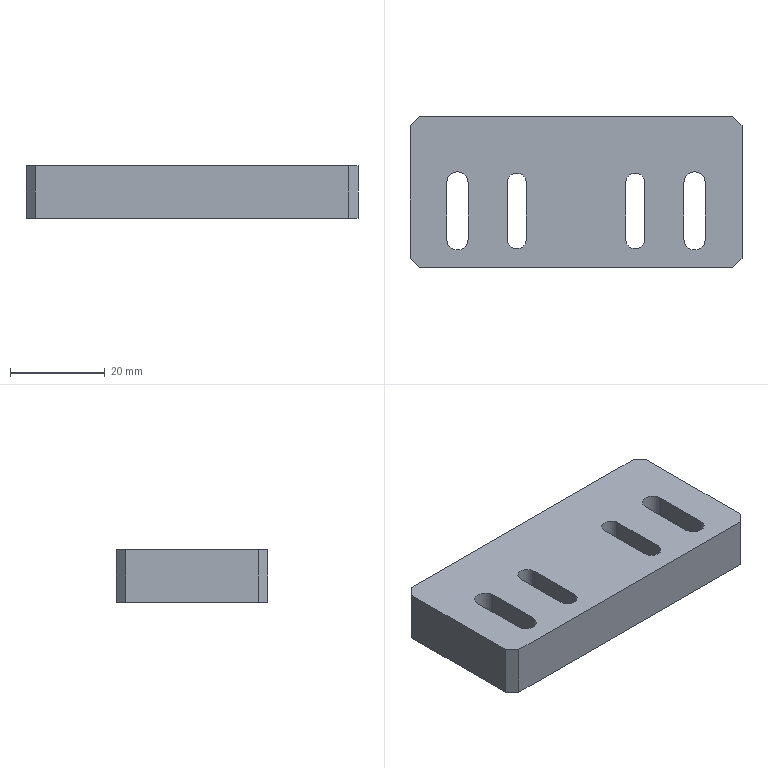Part | SolidWorks | features HoleWzd 4, Chamfer 1, Extrusion 1 | 1 solid | 46 faces | box 70 x 32 x 11 mm | volume 21010 mm3 | cylinder 18 | plane 18 | cone 10 | commonest cylinder face diameters 4 x8 4.2 x6 4.5 x4
STEP:
#1=CARTESIAN_POINT('',(-18.,10.,3.5));
#2=VERTEX_POINT('',#1);
#3=CARTESIAN_POINT('',(-18.,10.,7.5));
#4=VERTEX_POINT('',#3);
#5=CARTESIAN_POINT('',(-18.,10.,5.5));
#6=DIRECTION('',(0.,1.,0.));
#7=DIRECTION('',(0.,0.,1.));
#8=AXIS2_PLACEMENT_3D('',#5,#6,#7);
#9=CIRCLE('',#8,2.);
#10=EDGE_CURVE('',#2,#4,#9,.T.);
#11=ORIENTED_EDGE('',*,*,#10,.F.);
#12=CARTESIAN_POINT('',(-18.,16.,3.5));
#13=VERTEX_POINT('',#12);
#14=CARTESIAN_POINT('',(-18.,16.,3.5));
#15=DIRECTION('',(0.,1.,0.));
#16=VECTOR('',#15,1000.);
#17=LINE('',#14,#16);
#18=EDGE_CURVE('',#2,#13,#17,.T.);
#19=ORIENTED_EDGE('',*,*,#18,.T.);
#20=CARTESIAN_POINT('',(-18.,16.,7.5));
#21=VERTEX_POINT('',#20);
#22=CARTESIAN_POINT('',(-18.,16.,5.5));
#23=DIRECTION('',(0.,1.,0.));
#24=DIRECTION('',(0.,0.,1.));
#25=AXIS2_PLACEMENT_3D('',#22,#23,#24);
#26=CIRCLE('',#25,2.);
#27=EDGE_CURVE('',#13,#21,#26,.T.);
#28=ORIENTED_EDGE('',*,*,#27,.T.);
#29=CARTESIAN_POINT('',(-18.,16.,7.5));
#30=DIRECTION('',(0.,1.,0.));
#31=VECTOR('',#30,1000.);
#32=LINE('',#29,#31);
#33=EDGE_CURVE('',#4,#21,#32,.T.);
#34=ORIENTED_EDGE('',*,*,#33,.F.);
#35=EDGE_LOOP('',(#11,#19,#28,#34));
#36=FACE_OUTER_BOUND('',#35,.T.);
#37=CARTESIAN_POINT('',(-18.,16.,5.5));
#38=DIRECTION('',(0.,1.,0.));
#39=DIRECTION('',(0.,0.,1.));
#40=AXIS2_PLACEMENT_3D('',#37,#38,#39);
#41=CYLINDRICAL_SURFACE('',#40,2.);
#42=ADVANCED_FACE('',(#36),#41,.F.);
#43=CARTESIAN_POINT('',(-18.,8.798,5.5));
#44=VERTEX_POINT('',#43);
#45=CARTESIAN_POINT('',(-18.,10.,7.5));
#46=DIRECTION('',(0.,0.515,0.8572));
#47=VECTOR('',#46,1000.);
#48=LINE('',#45,#47);
#49=EDGE_CURVE('',#44,#4,#48,.T.);
#50=ORIENTED_EDGE('',*,*,#49,.F.);
#51=CARTESIAN_POINT('',(-18.,10.,3.5));
#52=DIRECTION('',(0.,0.515,-0.8572));
#53=VECTOR('',#52,1000.);
#54=LINE('',#51,#53);
#55=EDGE_CURVE('',#44,#2,#54,.T.);
#56=ORIENTED_EDGE('',*,*,#55,.T.);
#57=ORIENTED_EDGE('',*,*,#10,.T.);
#58=EDGE_LOOP('',(#50,#56,#57));
#59=FACE_OUTER_BOUND('',#58,.T.);
#60=CARTESIAN_POINT('',(-18.,10.,5.5));
#61=DIRECTION('',(0.,1.,0.));
#62=DIRECTION('',(0.,0.,1.));
#63=AXIS2_PLACEMENT_3D('',#60,#61,#62);
#64=CONICAL_SURFACE('',#63,2.,1.03);
#65=ADVANCED_FACE('',(#59),#64,.F.);
#66=CARTESIAN_POINT('',(18.,10.,3.5));
#67=VERTEX_POINT('',#66);
#68=CARTESIAN_POINT('',(18.,10.,7.5));
#69=VERTEX_POINT('',#68);
#70=CARTESIAN_POINT('',(18.,10.,5.5));
#71=DIRECTION('',(0.,1.,0.));
#72=DIRECTION('',(0.,0.,1.));
#73=AXIS2_PLACEMENT_3D('',#70,#71,#72);
#74=CIRCLE('',#73,2.);
#75=EDGE_CURVE('',#67,#69,#74,.T.);
#76=ORIENTED_EDGE('',*,*,#75,.F.);
#77=CARTESIAN_POINT('',(18.,16.,3.5));
#78=VERTEX_POINT('',#77);
#79=CARTESIAN_POINT('',(18.,16.,3.5));
#80=DIRECTION('',(0.,1.,0.));
#81=VECTOR('',#80,1000.);
#82=LINE('',#79,#81);
#83=EDGE_CURVE('',#67,#78,#82,.T.);
#84=ORIENTED_EDGE('',*,*,#83,.T.);
#85=CARTESIAN_POINT('',(18.,16.,7.5));
#86=VERTEX_POINT('',#85);
#87=CARTESIAN_POINT('',(18.,16.,5.5));
#88=DIRECTION('',(0.,1.,0.));
#89=DIRECTION('',(0.,0.,1.));
#90=AXIS2_PLACEMENT_3D('',#87,#88,#89);
#91=CIRCLE('',#90,2.);
#92=EDGE_CURVE('',#78,#86,#91,.T.);
#93=ORIENTED_EDGE('',*,*,#92,.T.);
#94=CARTESIAN_POINT('',(18.,16.,7.5));
#95=DIRECTION('',(0.,1.,0.));
#96=VECTOR('',#95,1000.);
#97=LINE('',#94,#96);
#98=EDGE_CURVE('',#69,#86,#97,.T.);
#99=ORIENTED_EDGE('',*,*,#98,.F.);
#100=EDGE_LOOP('',(#76,#84,#93,#99));
#101=FACE_OUTER_BOUND('',#100,.T.);
#102=CARTESIAN_POINT('',(18.,16.,5.5));
#103=DIRECTION('',(0.,1.,0.));
#104=DIRECTION('',(0.,0.,1.));
#105=AXIS2_PLACEMENT_3D('',#102,#103,#104);
#106=CYLINDRICAL_SURFACE('',#105,2.);
#107=ADVANCED_FACE('',(#101),#106,.F.);
#108=CARTESIAN_POINT('',(18.,8.798,5.5));
#109=VERTEX_POINT('',#108);
#110=CARTESIAN_POINT('',(18.,10.,7.5));
#111=DIRECTION('',(0.,0.515,0.8572));
#112=VECTOR('',#111,1000.);
#113=LINE('',#110,#112);
#114=EDGE_CURVE('',#109,#69,#113,.T.);
#115=ORIENTED_EDGE('',*,*,#114,.F.);
#116=CARTESIAN_POINT('',(18.,10.,3.5));
#117=DIRECTION('',(0.,0.515,-0.8572));
#118=VECTOR('',#117,1000.);
#119=LINE('',#116,#118);
#120=EDGE_CURVE('',#109,#67,#119,.T.);
#121=ORIENTED_EDGE('',*,*,#120,.T.);
#122=ORIENTED_EDGE('',*,*,#75,.T.);
#123=EDGE_LOOP('',(#115,#121,#122));
#124=FACE_OUTER_BOUND('',#123,.T.);
#125=CARTESIAN_POINT('',(18.,10.,5.5));
#126=DIRECTION('',(0.,1.,0.));
#127=DIRECTION('',(0.,0.,1.));
#128=AXIS2_PLACEMENT_3D('',#125,#126,#127);
#129=CONICAL_SURFACE('',#128,2.,1.03);
#130=ADVANCED_FACE('',(#124),#129,.F.);
#131=CARTESIAN_POINT('',(23.418,3.6,4.119));
#132=VERTEX_POINT('',#131);
#133=CARTESIAN_POINT('',(25.,4.25,3.4));
#134=VERTEX_POINT('',#133);
#135=CARTESIAN_POINT('',(23.418,3.6,4.119));
#136=CARTESIAN_POINT('',(23.508,3.688,4.016));
#137=CARTESIAN_POINT('',(23.607,3.772,3.922));
#138=CARTESIAN_POINT('',(23.83,3.927,3.75));
#139=CARTESIAN_POINT('',(23.955,3.998,3.672));
#140=CARTESIAN_POINT('',(24.225,4.117,3.542));
#141=CARTESIAN_POINT('',(24.371,4.166,3.49));
#142=CARTESIAN_POINT('',(24.68,4.233,3.418));
#143=CARTESIAN_POINT('',(24.838,4.25,3.4));
#144=CARTESIAN_POINT('',(25.,4.25,3.4));
#145=B_SPLINE_CURVE_WITH_KNOTS('',3,(#135,#136,#137,#138,#139,#140,#141,#142,#143,#144),.UNSPECIFIED.,.F.,.F.,(4,2,2,2,4),(0.,0.0004814,0.0009628,0.001444,0.001926),.UNSPECIFIED.);
#146=EDGE_CURVE('',#132,#134,#145,.T.);
#147=ORIENTED_EDGE('',*,*,#146,.T.);
#148=CARTESIAN_POINT('',(25.,16.,3.4));
#149=VERTEX_POINT('',#148);
#150=CARTESIAN_POINT('',(25.,16.,3.4));
#151=DIRECTION('',(0.,1.,0.));
#152=VECTOR('',#151,1000.);
#153=LINE('',#150,#152);
#154=EDGE_CURVE('',#134,#149,#153,.T.);
#155=ORIENTED_EDGE('',*,*,#154,.T.);
#156=CARTESIAN_POINT('',(25.,16.,7.6));
#157=VERTEX_POINT('',#156);
#158=CARTESIAN_POINT('',(25.,16.,5.5));
#159=DIRECTION('',(0.,1.,0.));
#160=DIRECTION('',(0.,0.,1.));
#161=AXIS2_PLACEMENT_3D('',#158,#159,#160);
#162=CIRCLE('',#161,2.1);
#163=EDGE_CURVE('',#149,#157,#162,.T.);
#164=ORIENTED_EDGE('',*,*,#163,.T.);
#165=CARTESIAN_POINT('',(25.,4.25,7.6));
#166=VERTEX_POINT('',#165);
#167=CARTESIAN_POINT('',(25.,16.,7.6));
#168=DIRECTION('',(0.,1.,0.));
#169=VECTOR('',#168,1000.);
#170=LINE('',#167,#169);
#171=EDGE_CURVE('',#166,#157,#170,.T.);
#172=ORIENTED_EDGE('',*,*,#171,.F.);
#173=CARTESIAN_POINT('',(23.418,3.6,6.881));
#174=VERTEX_POINT('',#173);
#175=CARTESIAN_POINT('',(25.,4.25,7.6));
#176=CARTESIAN_POINT('',(24.677,4.25,7.6));
#177=CARTESIAN_POINT('',(24.358,4.177,7.522));
#178=CARTESIAN_POINT('',(23.954,3.997,7.327));
#179=CARTESIAN_POINT('',(23.829,3.926,7.249));
#180=CARTESIAN_POINT('',(23.607,3.772,7.078));
#181=CARTESIAN_POINT('',(23.507,3.688,6.983));
#182=CARTESIAN_POINT('',(23.418,3.6,6.881));
#183=B_SPLINE_CURVE_WITH_KNOTS('',3,(#175,#176,#177,#178,#179,#180,#181,#182),.UNSPECIFIED.,.F.,.F.,(4,2,2,4),(0.001926,0.002886,0.003366,0.003846),.UNSPECIFIED.);
#184=EDGE_CURVE('',#166,#174,#183,.T.);
#185=ORIENTED_EDGE('',*,*,#184,.T.);
#186=CARTESIAN_POINT('',(25.,3.6,5.5));
#187=DIRECTION('',(0.,1.,0.));
#188=DIRECTION('',(0.,0.,1.));
#189=AXIS2_PLACEMENT_3D('',#186,#187,#188);
#190=CIRCLE('',#189,2.1);
#191=EDGE_CURVE('',#132,#174,#190,.T.);
#192=ORIENTED_EDGE('',*,*,#191,.F.);
#193=EDGE_LOOP('',(#147,#155,#164,#172,#185,#192));
#194=FACE_OUTER_BOUND('',#193,.T.);
#195=CARTESIAN_POINT('',(25.,16.,5.5));
#196=DIRECTION('',(0.,1.,0.));
#197=DIRECTION('',(0.,0.,1.));
#198=AXIS2_PLACEMENT_3D('',#195,#196,#197);
#199=CYLINDRICAL_SURFACE('',#198,2.1);
#200=ADVANCED_FACE('',(#194),#199,.F.);
#201=CARTESIAN_POINT('',(0.,3.6,3.4));
#202=VERTEX_POINT('',#201);
#203=CARTESIAN_POINT('',(0.,3.6,7.6));
#204=VERTEX_POINT('',#203);
#205=CARTESIAN_POINT('',(0.,3.6,5.5));
#206=DIRECTION('',(0.,1.,0.));
#207=DIRECTION('',(0.,0.,1.));
#208=AXIS2_PLACEMENT_3D('',#205,#206,#207);
#209=CIRCLE('',#208,2.1);
#210=EDGE_CURVE('',#202,#204,#209,.T.);
#211=ORIENTED_EDGE('',*,*,#210,.F.);
#212=CARTESIAN_POINT('',(0.,16.,3.4));
#213=VERTEX_POINT('',#212);
#214=CARTESIAN_POINT('',(0.,16.,3.4));
#215=DIRECTION('',(0.,1.,0.));
#216=VECTOR('',#215,1000.);
#217=LINE('',#214,#216);
#218=EDGE_CURVE('',#202,#213,#217,.T.);
#219=ORIENTED_EDGE('',*,*,#218,.T.);
#220=CARTESIAN_POINT('',(0.,16.,7.6));
#221=VERTEX_POINT('',#220);
#222=CARTESIAN_POINT('',(0.,16.,5.5));
#223=DIRECTION('',(0.,1.,0.));
#224=DIRECTION('',(0.,0.,1.));
#225=AXIS2_PLACEMENT_3D('',#222,#223,#224);
#226=CIRCLE('',#225,2.1);
#227=EDGE_CURVE('',#213,#221,#226,.T.);
#228=ORIENTED_EDGE('',*,*,#227,.T.);
#229=CARTESIAN_POINT('',(0.,16.,7.6));
#230=DIRECTION('',(0.,1.,0.));
#231=VECTOR('',#230,1000.);
#232=LINE('',#229,#231);
#233=EDGE_CURVE('',#204,#221,#232,.T.);
#234=ORIENTED_EDGE('',*,*,#233,.F.);
#235=EDGE_LOOP('',(#211,#219,#228,#234));
#236=FACE_OUTER_BOUND('',#235,.T.);
#237=CARTESIAN_POINT('',(0.,16.,5.5));
#238=DIRECTION('',(0.,1.,0.));
#239=DIRECTION('',(0.,0.,1.));
#240=AXIS2_PLACEMENT_3D('',#237,#238,#239);
#241=CYLINDRICAL_SURFACE('',#240,2.1);
#242=ADVANCED_FACE('',(#236),#241,.F.);
#243=CARTESIAN_POINT('',(0.,2.338,5.5));
#244=VERTEX_POINT('',#243);
#245=CARTESIAN_POINT('',(0.,3.6,7.6));
#246=DIRECTION('',(0.,0.515,0.8572));
#247=VECTOR('',#246,1000.);
#248=LINE('',#245,#247);
#249=EDGE_CURVE('',#244,#204,#248,.T.);
#250=ORIENTED_EDGE('',*,*,#249,.F.);
#251=CARTESIAN_POINT('',(0.,3.6,3.4));
#252=DIRECTION('',(0.,0.515,-0.8572));
#253=VECTOR('',#252,1000.);
#254=LINE('',#251,#253);
#255=EDGE_CURVE('',#244,#202,#254,.T.);
#256=ORIENTED_EDGE('',*,*,#255,.T.);
#257=ORIENTED_EDGE('',*,*,#210,.T.);
#258=EDGE_LOOP('',(#250,#256,#257));
#259=FACE_OUTER_BOUND('',#258,.T.);
#260=CARTESIAN_POINT('',(0.,3.6,5.5));
#261=DIRECTION('',(0.,1.,0.));
#262=DIRECTION('',(0.,0.,1.));
#263=AXIS2_PLACEMENT_3D('',#260,#261,#262);
#264=CONICAL_SURFACE('',#263,2.1,1.03);
#265=ADVANCED_FACE('',(#259),#264,.F.);
#266=CARTESIAN_POINT('',(-26.582,3.6,4.119));
#267=VERTEX_POINT('',#266);
#268=CARTESIAN_POINT('',(-25.,4.25,3.4));
#269=VERTEX_POINT('',#268);
#270=CARTESIAN_POINT('',(-26.582,3.6,4.119));
#271=CARTESIAN_POINT('',(-26.492,3.688,4.016));
#272=CARTESIAN_POINT('',(-26.393,3.772,3.922));
#273=CARTESIAN_POINT('',(-26.17,3.927,3.75));
#274=CARTESIAN_POINT('',(-26.045,3.998,3.672));
#275=CARTESIAN_POINT('',(-25.775,4.117,3.542));
#276=CARTESIAN_POINT('',(-25.629,4.166,3.49));
#277=CARTESIAN_POINT('',(-25.32,4.233,3.418));
#278=CARTESIAN_POINT('',(-25.162,4.25,3.4));
#279=CARTESIAN_POINT('',(-25.,4.25,3.4));
#280=B_SPLINE_CURVE_WITH_KNOTS('',3,(#270,#271,#272,#273,#274,#275,#276,#277,#278,#279),.UNSPECIFIED.,.F.,.F.,(4,2,2,2,4),(0.,0.0004814,0.0009628,0.001444,0.001926),.UNSPECIFIED.);
#281=EDGE_CURVE('',#267,#269,#280,.T.);
#282=ORIENTED_EDGE('',*,*,#281,.T.);
#283=CARTESIAN_POINT('',(-25.,16.,3.4));
#284=VERTEX_POINT('',#283);
#285=CARTESIAN_POINT('',(-25.,16.,3.4));
#286=DIRECTION('',(0.,1.,0.));
#287=VECTOR('',#286,1000.);
#288=LINE('',#285,#287);
#289=EDGE_CURVE('',#269,#284,#288,.T.);
#290=ORIENTED_EDGE('',*,*,#289,.T.);
#291=CARTESIAN_POINT('',(-25.,16.,7.6));
#292=VERTEX_POINT('',#291);
#293=CARTESIAN_POINT('',(-25.,16.,5.5));
#294=DIRECTION('',(0.,1.,0.));
#295=DIRECTION('',(0.,0.,1.));
#296=AXIS2_PLACEMENT_3D('',#293,#294,#295);
#297=CIRCLE('',#296,2.1);
#298=EDGE_CURVE('',#284,#292,#297,.T.);
#299=ORIENTED_EDGE('',*,*,#298,.T.);
#300=CARTESIAN_POINT('',(-25.,4.25,7.6));
#301=VERTEX_POINT('',#300);
#302=CARTESIAN_POINT('',(-25.,16.,7.6));
#303=DIRECTION('',(0.,1.,0.));
#304=VECTOR('',#303,1000.);
#305=LINE('',#302,#304);
#306=EDGE_CURVE('',#301,#292,#305,.T.);
#307=ORIENTED_EDGE('',*,*,#306,.F.);
#308=CARTESIAN_POINT('',(-26.582,3.6,6.881));
#309=VERTEX_POINT('',#308);
#310=CARTESIAN_POINT('',(-25.,4.25,7.6));
#311=CARTESIAN_POINT('',(-25.323,4.25,7.6));
#312=CARTESIAN_POINT('',(-25.642,4.177,7.522));
#313=CARTESIAN_POINT('',(-26.046,3.997,7.327));
#314=CARTESIAN_POINT('',(-26.171,3.926,7.249));
#315=CARTESIAN_POINT('',(-26.393,3.772,7.078));
#316=CARTESIAN_POINT('',(-26.493,3.688,6.983));
#317=CARTESIAN_POINT('',(-26.582,3.6,6.881));
#318=B_SPLINE_CURVE_WITH_KNOTS('',3,(#310,#311,#312,#313,#314,#315,#316,#317),.UNSPECIFIED.,.F.,.F.,(4,2,2,4),(0.001926,0.002886,0.003366,0.003846),.UNSPECIFIED.);
#319=EDGE_CURVE('',#301,#309,#318,.T.);
#320=ORIENTED_EDGE('',*,*,#319,.T.);
#321=CARTESIAN_POINT('',(-25.,3.6,5.5));
#322=DIRECTION('',(0.,1.,0.));
#323=DIRECTION('',(0.,0.,1.));
#324=AXIS2_PLACEMENT_3D('',#321,#322,#323);
#325=CIRCLE('',#324,2.1);
#326=EDGE_CURVE('',#267,#309,#325,.T.);
#327=ORIENTED_EDGE('',*,*,#326,.F.);
#328=EDGE_LOOP('',(#282,#290,#299,#307,#320,#327));
#329=FACE_OUTER_BOUND('',#328,.T.);
#330=CARTESIAN_POINT('',(-25.,16.,5.5));
#331=DIRECTION('',(0.,1.,0.));
#332=DIRECTION('',(0.,0.,1.));
#333=AXIS2_PLACEMENT_3D('',#330,#331,#332);
#334=CYLINDRICAL_SURFACE('',#333,2.1);
#335=ADVANCED_FACE('',(#329),#334,.F.);
#336=CARTESIAN_POINT('',(27.25,-10.,0.));
#337=VERTEX_POINT('',#336);
#338=CARTESIAN_POINT('',(27.25,2.,0.));
#339=VERTEX_POINT('',#338);
#340=CARTESIAN_POINT('',(27.25,-10.,0.));
#341=DIRECTION('',(0.,1.,0.));
#342=VECTOR('',#341,1000.);
#343=LINE('',#340,#342);
#344=EDGE_CURVE('',#337,#339,#343,.T.);
#345=ORIENTED_EDGE('',*,*,#344,.T.);
#346=CARTESIAN_POINT('',(22.75,2.,0.));
#347=VERTEX_POINT('',#346);
#348=CARTESIAN_POINT('',(25.,2.,0.));
#349=DIRECTION('',(0.,0.,-1.));
#350=DIRECTION('',(-1.,0.,0.));
#351=AXIS2_PLACEMENT_3D('',#348,#349,#350);
#352=CIRCLE('',#351,2.25);
#353=EDGE_CURVE('',#347,#339,#352,.T.);
#354=ORIENTED_EDGE('',*,*,#353,.F.);
#355=CARTESIAN_POINT('',(22.75,-10.,0.));
#356=VERTEX_POINT('',#355);
#357=CARTESIAN_POINT('',(22.75,-10.,0.));
#358=DIRECTION('',(0.,1.,0.));
#359=VECTOR('',#358,1000.);
#360=LINE('',#357,#359);
#361=EDGE_CURVE('',#356,#347,#360,.T.);
#362=ORIENTED_EDGE('',*,*,#361,.F.);
#363=CARTESIAN_POINT('',(25.,-10.,0.));
#364=DIRECTION('',(0.,0.,-1.));
#365=DIRECTION('',(-1.,0.,0.));
#366=AXIS2_PLACEMENT_3D('',#363,#364,#365);
#367=CIRCLE('',#366,2.25);
#368=EDGE_CURVE('',#337,#356,#367,.T.);
#369=ORIENTED_EDGE('',*,*,#368,.F.);
#370=EDGE_LOOP('',(#345,#354,#362,#369));
#371=FACE_BOUND('',#370,.T.);
#372=CARTESIAN_POINT('',(35.,-14.,0.));
#373=VERTEX_POINT('',#372);
#374=CARTESIAN_POINT('',(35.,14.,0.));
#375=VERTEX_POINT('',#374);
#376=CARTESIAN_POINT('',(35.,16.,0.));
#377=DIRECTION('',(0.,1.,0.));
#378=VECTOR('',#377,1000.);
#379=LINE('',#376,#378);
#380=EDGE_CURVE('',#373,#375,#379,.T.);
#381=ORIENTED_EDGE('',*,*,#380,.F.);
#382=CARTESIAN_POINT('',(33.,-16.,0.));
#383=VERTEX_POINT('',#382);
#384=CARTESIAN_POINT('',(35.,-14.,0.));
#385=DIRECTION('',(-0.7071,-0.7071,0.));
#386=VECTOR('',#385,1000.);
#387=LINE('',#384,#386);
#388=EDGE_CURVE('',#373,#383,#387,.T.);
#389=ORIENTED_EDGE('',*,*,#388,.T.);
#390=CARTESIAN_POINT('',(-33.,-16.,0.));
#391=VERTEX_POINT('',#390);
#392=CARTESIAN_POINT('',(-35.,-16.,0.));
#393=DIRECTION('',(1.,0.,0.));
#394=VECTOR('',#393,1000.);
#395=LINE('',#392,#394);
#396=EDGE_CURVE('',#391,#383,#395,.T.);
#397=ORIENTED_EDGE('',*,*,#396,.F.);
#398=CARTESIAN_POINT('',(-35.,-14.,0.));
#399=VERTEX_POINT('',#398);
#400=CARTESIAN_POINT('',(-33.,-16.,0.));
#401=DIRECTION('',(-0.7071,0.7071,0.));
#402=VECTOR('',#401,1000.);
#403=LINE('',#400,#402);
#404=EDGE_CURVE('',#391,#399,#403,.T.);
#405=ORIENTED_EDGE('',*,*,#404,.T.);
#406=CARTESIAN_POINT('',(-35.,14.,0.));
#407=VERTEX_POINT('',#406);
#408=CARTESIAN_POINT('',(-35.,16.,0.));
#409=DIRECTION('',(0.,-1.,0.));
#410=VECTOR('',#409,1000.);
#411=LINE('',#408,#410);
#412=EDGE_CURVE('',#407,#399,#411,.T.);
#413=ORIENTED_EDGE('',*,*,#412,.F.);
#414=CARTESIAN_POINT('',(-33.,16.,0.));
#415=VERTEX_POINT('',#414);
#416=CARTESIAN_POINT('',(-35.,14.,0.));
#417=DIRECTION('',(0.7071,0.7071,0.));
#418=VECTOR('',#417,1000.);
#419=LINE('',#416,#418);
#420=EDGE_CURVE('',#407,#415,#419,.T.);
#421=ORIENTED_EDGE('',*,*,#420,.T.);
#422=CARTESIAN_POINT('',(33.,16.,0.));
#423=VERTEX_POINT('',#422);
#424=CARTESIAN_POINT('',(-35.,16.,0.));
#425=DIRECTION('',(-1.,0.,0.));
#426=VECTOR('',#425,1000.);
#427=LINE('',#424,#426);
#428=EDGE_CURVE('',#423,#415,#427,.T.);
#429=ORIENTED_EDGE('',*,*,#428,.F.);
#430=CARTESIAN_POINT('',(33.,16.,0.));
#431=DIRECTION('',(0.7071,-0.7071,0.));
#432=VECTOR('',#431,1000.);
#433=LINE('',#430,#432);
#434=EDGE_CURVE('',#423,#375,#433,.T.);
#435=ORIENTED_EDGE('',*,*,#434,.T.);
#436=EDGE_LOOP('',(#381,#389,#397,#405,#413,#421,#429,#435));
#437=FACE_OUTER_BOUND('',#436,.T.);
#438=CARTESIAN_POINT('',(-27.25,2.,0.));
#439=VERTEX_POINT('',#438);
#440=CARTESIAN_POINT('',(-22.75,2.,0.));
#441=VERTEX_POINT('',#440);
#442=CARTESIAN_POINT('',(-25.,2.,0.));
#443=DIRECTION('',(0.,0.,-1.));
#444=DIRECTION('',(-1.,0.,0.));
#445=AXIS2_PLACEMENT_3D('',#442,#443,#444);
#446=CIRCLE('',#445,2.25);
#447=EDGE_CURVE('',#439,#441,#446,.T.);
#448=ORIENTED_EDGE('',*,*,#447,.F.);
#449=CARTESIAN_POINT('',(-27.25,-10.,0.));
#450=VERTEX_POINT('',#449);
#451=CARTESIAN_POINT('',(-27.25,-10.,0.));
#452=DIRECTION('',(0.,1.,0.));
#453=VECTOR('',#452,1000.);
#454=LINE('',#451,#453);
#455=EDGE_CURVE('',#450,#439,#454,.T.);
#456=ORIENTED_EDGE('',*,*,#455,.F.);
#457=CARTESIAN_POINT('',(-22.75,-10.,0.));
#458=VERTEX_POINT('',#457);
#459=CARTESIAN_POINT('',(-25.,-10.,0.));
#460=DIRECTION('',(0.,0.,-1.));
#461=DIRECTION('',(-1.,0.,0.));
#462=AXIS2_PLACEMENT_3D('',#459,#460,#461);
#463=CIRCLE('',#462,2.25);
#464=EDGE_CURVE('',#458,#450,#463,.T.);
#465=ORIENTED_EDGE('',*,*,#464,.F.);
#466=CARTESIAN_POINT('',(-22.75,-10.,0.));
#467=DIRECTION('',(0.,1.,0.));
#468=VECTOR('',#467,1000.);
#469=LINE('',#466,#468);
#470=EDGE_CURVE('',#458,#441,#469,.T.);
#471=ORIENTED_EDGE('',*,*,#470,.T.);
#472=EDGE_LOOP('',(#448,#456,#465,#471));
#473=FACE_BOUND('',#472,.T.);
#474=CARTESIAN_POINT('',(-14.5,2.,0.));
#475=VERTEX_POINT('',#474);
#476=CARTESIAN_POINT('',(-10.5,2.,0.));
#477=VERTEX_POINT('',#476);
#478=CARTESIAN_POINT('',(-12.5,2.,0.));
#479=DIRECTION('',(0.,0.,-1.));
#480=DIRECTION('',(-1.,0.,0.));
#481=AXIS2_PLACEMENT_3D('',#478,#479,#480);
#482=CIRCLE('',#481,2.);
#483=EDGE_CURVE('',#475,#477,#482,.T.);
#484=ORIENTED_EDGE('',*,*,#483,.F.);
#485=CARTESIAN_POINT('',(-14.5,-10.,0.));
#486=VERTEX_POINT('',#485);
#487=CARTESIAN_POINT('',(-14.5,-10.,0.));
#488=DIRECTION('',(0.,1.,0.));
#489=VECTOR('',#488,1000.);
#490=LINE('',#487,#489);
#491=EDGE_CURVE('',#486,#475,#490,.T.);
#492=ORIENTED_EDGE('',*,*,#491,.F.);
#493=CARTESIAN_POINT('',(-10.5,-10.,0.));
#494=VERTEX_POINT('',#493);
#495=CARTESIAN_POINT('',(-12.5,-10.,0.));
#496=DIRECTION('',(0.,0.,-1.));
#497=DIRECTION('',(-1.,0.,0.));
#498=AXIS2_PLACEMENT_3D('',#495,#496,#497);
#499=CIRCLE('',#498,2.);
#500=EDGE_CURVE('',#494,#486,#499,.T.);
#501=ORIENTED_EDGE('',*,*,#500,.F.);
#502=CARTESIAN_POINT('',(-10.5,-10.,0.));
#503=DIRECTION('',(0.,1.,0.));
#504=VECTOR('',#503,1000.);
#505=LINE('',#502,#504);
#506=EDGE_CURVE('',#494,#477,#505,.T.);
#507=ORIENTED_EDGE('',*,*,#506,.T.);
#508=EDGE_LOOP('',(#484,#492,#501,#507));
#509=FACE_BOUND('',#508,.T.);
#510=CARTESIAN_POINT('',(10.5,2.,0.));
#511=VERTEX_POINT('',#510);
#512=CARTESIAN_POINT('',(14.5,2.,0.));
#513=VERTEX_POINT('',#512);
#514=CARTESIAN_POINT('',(12.5,2.,0.));
#515=DIRECTION('',(0.,0.,-1.));
#516=DIRECTION('',(-1.,0.,0.));
#517=AXIS2_PLACEMENT_3D('',#514,#515,#516);
#518=CIRCLE('',#517,2.);
#519=EDGE_CURVE('',#511,#513,#518,.T.);
#520=ORIENTED_EDGE('',*,*,#519,.F.);
#521=CARTESIAN_POINT('',(10.5,-10.,0.));
#522=VERTEX_POINT('',#521);
#523=CARTESIAN_POINT('',(10.5,-10.,0.));
#524=DIRECTION('',(0.,1.,0.));
#525=VECTOR('',#524,1000.);
#526=LINE('',#523,#525);
#527=EDGE_CURVE('',#522,#511,#526,.T.);
#528=ORIENTED_EDGE('',*,*,#527,.F.);
#529=CARTESIAN_POINT('',(14.5,-10.,0.));
#530=VERTEX_POINT('',#529);
#531=CARTESIAN_POINT('',(12.5,-10.,0.));
#532=DIRECTION('',(0.,0.,-1.));
#533=DIRECTION('',(-1.,0.,0.));
#534=AXIS2_PLACEMENT_3D('',#531,#532,#533);
#535=CIRCLE('',#534,2.);
#536=EDGE_CURVE('',#530,#522,#535,.T.);
#537=ORIENTED_EDGE('',*,*,#536,.F.);
#538=CARTESIAN_POINT('',(14.5,-10.,0.));
#539=DIRECTION('',(0.,1.,0.));
#540=VECTOR('',#539,1000.);
#541=LINE('',#538,#540);
#542=EDGE_CURVE('',#530,#513,#541,.T.);
#543=ORIENTED_EDGE('',*,*,#542,.T.);
#544=EDGE_LOOP('',(#520,#528,#537,#543));
#545=FACE_BOUND('',#544,.T.);
#546=CARTESIAN_POINT('',(0.,0.,0.));
#547=DIRECTION('',(0.,0.,1.));
#548=DIRECTION('',(1.,0.,0.));
#549=AXIS2_PLACEMENT_3D('',#546,#547,#548);
#550=PLANE('',#549);
#551=ADVANCED_FACE('',(#371,#437,#473,#509,#545),#550,.F.);
#552=ORIENTED_EDGE('',*,*,#191,.T.);
#553=CARTESIAN_POINT('',(23.418,3.6,6.881));
#554=CARTESIAN_POINT('',(23.358,3.54,6.661));
#555=CARTESIAN_POINT('',(23.313,3.489,6.436));
#556=CARTESIAN_POINT('',(23.252,3.417,5.971));
#557=CARTESIAN_POINT('',(23.237,3.398,5.735));
#558=CARTESIAN_POINT('',(23.237,3.398,5.265));
#559=CARTESIAN_POINT('',(23.252,3.417,5.028));
#560=CARTESIAN_POINT('',(23.313,3.489,4.564));
#561=CARTESIAN_POINT('',(23.358,3.54,4.339));
#562=CARTESIAN_POINT('',(23.418,3.6,4.119));
#563=B_SPLINE_CURVE_WITH_KNOTS('',3,(#553,#554,#555,#556,#557,#558,#559,#560,#561,#562),.UNSPECIFIED.,.F.,.F.,(4,2,2,2,4),(0.000461,0.001167,0.001873,0.002579,0.003285),.UNSPECIFIED.);
#564=EDGE_CURVE('',#174,#132,#563,.T.);
#565=ORIENTED_EDGE('',*,*,#564,.T.);
#566=EDGE_LOOP('',(#552,#565));
#567=FACE_OUTER_BOUND('',#566,.T.);
#568=CARTESIAN_POINT('',(25.,3.6,5.5));
#569=DIRECTION('',(0.,1.,0.));
#570=DIRECTION('',(0.,0.,1.));
#571=AXIS2_PLACEMENT_3D('',#568,#569,#570);
#572=CONICAL_SURFACE('',#571,2.1,1.03);
#573=ADVANCED_FACE('',(#567),#572,.F.);
#574=ORIENTED_EDGE('',*,*,#326,.T.);
#575=CARTESIAN_POINT('',(-26.582,3.6,6.881));
#576=CARTESIAN_POINT('',(-26.642,3.54,6.661));
#577=CARTESIAN_POINT('',(-26.687,3.489,6.436));
#578=CARTESIAN_POINT('',(-26.748,3.417,5.971));
#579=CARTESIAN_POINT('',(-26.763,3.398,5.735));
#580=CARTESIAN_POINT('',(-26.763,3.398,5.265));
#581=CARTESIAN_POINT('',(-26.748,3.417,5.028));
#582=CARTESIAN_POINT('',(-26.687,3.489,4.564));
#583=CARTESIAN_POINT('',(-26.642,3.54,4.339));
#584=CARTESIAN_POINT('',(-26.582,3.6,4.119));
#585=B_SPLINE_CURVE_WITH_KNOTS('',3,(#575,#576,#577,#578,#579,#580,#581,#582,#583,#584),.UNSPECIFIED.,.F.,.F.,(4,2,2,2,4),(0.000461,0.001167,0.001873,0.002579,0.003285),.UNSPECIFIED.);
#586=EDGE_CURVE('',#309,#267,#585,.T.);
#587=ORIENTED_EDGE('',*,*,#586,.T.);
#588=EDGE_LOOP('',(#574,#587));
#589=FACE_OUTER_BOUND('',#588,.T.);
#590=CARTESIAN_POINT('',(-25.,3.6,5.5));
#591=DIRECTION('',(0.,1.,0.));
#592=DIRECTION('',(0.,0.,1.));
#593=AXIS2_PLACEMENT_3D('',#590,#591,#592);
#594=CONICAL_SURFACE('',#593,2.1,1.03);
#595=ADVANCED_FACE('',(#589),#594,.F.);
#596=CARTESIAN_POINT('',(35.,-14.,11.));
#597=VERTEX_POINT('',#596);
#598=CARTESIAN_POINT('',(35.,14.,11.));
#599=VERTEX_POINT('',#598);
#600=CARTESIAN_POINT('',(35.,16.,11.));
#601=DIRECTION('',(0.,1.,0.));
#602=VECTOR('',#601,1000.);
#603=LINE('',#600,#602);
#604=EDGE_CURVE('',#597,#599,#603,.T.);
#605=ORIENTED_EDGE('',*,*,#604,.F.);
#606=CARTESIAN_POINT('',(35.,-14.,11.));
#607=DIRECTION('',(0.,0.,-1.));
#608=VECTOR('',#607,1000.);
#609=LINE('',#606,#608);
#610=EDGE_CURVE('',#597,#373,#609,.T.);
#611=ORIENTED_EDGE('',*,*,#610,.T.);
#612=ORIENTED_EDGE('',*,*,#380,.T.);
#613=CARTESIAN_POINT('',(35.,14.,11.));
#614=DIRECTION('',(0.,0.,1.));
#615=VECTOR('',#614,1000.);
#616=LINE('',#613,#615);
#617=EDGE_CURVE('',#375,#599,#616,.T.);
#618=ORIENTED_EDGE('',*,*,#617,.T.);
#619=EDGE_LOOP('',(#605,#611,#612,#618));
#620=FACE_OUTER_BOUND('',#619,.T.);
#621=CARTESIAN_POINT('',(35.,16.,11.));
#622=DIRECTION('',(-1.,0.,0.));
#623=DIRECTION('',(0.,-1.,0.));
#624=AXIS2_PLACEMENT_3D('',#621,#622,#623);
#625=PLANE('',#624);
#626=ADVANCED_FACE('',(#620),#625,.F.);
#627=CARTESIAN_POINT('',(-18.,16.,5.5));
#628=DIRECTION('',(0.,1.,0.));
#629=DIRECTION('',(0.,0.,1.));
#630=AXIS2_PLACEMENT_3D('',#627,#628,#629);
#631=CIRCLE('',#630,2.);
#632=EDGE_CURVE('',#21,#13,#631,.T.);
#633=ORIENTED_EDGE('',*,*,#632,.F.);
#634=ORIENTED_EDGE('',*,*,#27,.F.);
#635=EDGE_LOOP('',(#633,#634));
#636=FACE_BOUND('',#635,.T.);
#637=CARTESIAN_POINT('',(18.,16.,5.5));
#638=DIRECTION('',(0.,1.,0.));
#639=DIRECTION('',(0.,0.,1.));
#640=AXIS2_PLACEMENT_3D('',#637,#638,#639);
#641=CIRCLE('',#640,2.);
#642=EDGE_CURVE('',#86,#78,#641,.T.);
#643=ORIENTED_EDGE('',*,*,#642,.F.);
#644=ORIENTED_EDGE('',*,*,#92,.F.);
#645=EDGE_LOOP('',(#643,#644));
#646=FACE_BOUND('',#645,.T.);
#647=CARTESIAN_POINT('',(25.,16.,5.5));
#648=DIRECTION('',(0.,1.,0.));
#649=DIRECTION('',(0.,0.,1.));
#650=AXIS2_PLACEMENT_3D('',#647,#648,#649);
#651=CIRCLE('',#650,2.1);
#652=EDGE_CURVE('',#157,#149,#651,.T.);
#653=ORIENTED_EDGE('',*,*,#652,.F.);
#654=ORIENTED_EDGE('',*,*,#163,.F.);
#655=EDGE_LOOP('',(#653,#654));
#656=FACE_BOUND('',#655,.T.);
#657=CARTESIAN_POINT('',(0.,16.,5.5));
#658=DIRECTION('',(0.,1.,0.));
#659=DIRECTION('',(0.,0.,1.));
#660=AXIS2_PLACEMENT_3D('',#657,#658,#659);
#661=CIRCLE('',#660,2.1);
#662=EDGE_CURVE('',#221,#213,#661,.T.);
#663=ORIENTED_EDGE('',*,*,#662,.F.);
#664=ORIENTED_EDGE('',*,*,#227,.F.);
#665=EDGE_LOOP('',(#663,#664));
#666=FACE_BOUND('',#665,.T.);
#667=CARTESIAN_POINT('',(-25.,16.,5.5));
#668=DIRECTION('',(0.,1.,0.));
#669=DIRECTION('',(0.,0.,1.));
#670=AXIS2_PLACEMENT_3D('',#667,#668,#669);
#671=CIRCLE('',#670,2.1);
#672=EDGE_CURVE('',#292,#284,#671,.T.);
#673=ORIENTED_EDGE('',*,*,#672,.F.);
#674=ORIENTED_EDGE('',*,*,#298,.F.);
#675=EDGE_LOOP('',(#673,#674));
#676=FACE_BOUND('',#675,.T.);
#677=CARTESIAN_POINT('',(33.,16.,11.));
#678=VERTEX_POINT('',#677);
#679=CARTESIAN_POINT('',(-33.,16.,11.));
#680=VERTEX_POINT('',#679);
#681=CARTESIAN_POINT('',(-35.,16.,11.));
#682=DIRECTION('',(-1.,0.,0.));
#683=VECTOR('',#682,1000.);
#684=LINE('',#681,#683);
#685=EDGE_CURVE('',#678,#680,#684,.T.);
#686=ORIENTED_EDGE('',*,*,#685,.F.);
#687=CARTESIAN_POINT('',(33.,16.,11.));
#688=DIRECTION('',(0.,0.,-1.));
#689=VECTOR('',#688,1000.);
#690=LINE('',#687,#689);
#691=EDGE_CURVE('',#678,#423,#690,.T.);
#692=ORIENTED_EDGE('',*,*,#691,.T.);
#693=ORIENTED_EDGE('',*,*,#428,.T.);
#694=CARTESIAN_POINT('',(-33.,16.,11.));
#695=DIRECTION('',(0.,0.,1.));
#696=VECTOR('',#695,1000.);
#697=LINE('',#694,#696);
#698=EDGE_CURVE('',#415,#680,#697,.T.);
#699=ORIENTED_EDGE('',*,*,#698,.T.);
#700=EDGE_LOOP('',(#686,#692,#693,#699));
#701=FACE_OUTER_BOUND('',#700,.T.);
#702=CARTESIAN_POINT('',(-35.,16.,11.));
#703=DIRECTION('',(0.,-1.,0.));
#704=DIRECTION('',(0.,0.,-1.));
#705=AXIS2_PLACEMENT_3D('',#702,#703,#704);
#706=PLANE('',#705);
#707=ADVANCED_FACE('',(#636,#646,#656,#666,#676,#701),#706,.F.);
#708=CARTESIAN_POINT('',(-35.,14.,11.));
#709=VERTEX_POINT('',#708);
#710=CARTESIAN_POINT('',(-35.,-14.,11.));
#711=VERTEX_POINT('',#710);
#712=CARTESIAN_POINT('',(-35.,16.,11.));
#713=DIRECTION('',(0.,-1.,0.));
#714=VECTOR('',#713,1000.);
#715=LINE('',#712,#714);
#716=EDGE_CURVE('',#709,#711,#715,.T.);
#717=ORIENTED_EDGE('',*,*,#716,.F.);
#718=CARTESIAN_POINT('',(-35.,14.,11.));
#719=DIRECTION('',(0.,0.,-1.));
#720=VECTOR('',#719,1000.);
#721=LINE('',#718,#720);
#722=EDGE_CURVE('',#709,#407,#721,.T.);
#723=ORIENTED_EDGE('',*,*,#722,.T.);
#724=ORIENTED_EDGE('',*,*,#412,.T.);
#725=CARTESIAN_POINT('',(-35.,-14.,11.));
#726=DIRECTION('',(0.,0.,1.));
#727=VECTOR('',#726,1000.);
#728=LINE('',#725,#727);
#729=EDGE_CURVE('',#399,#711,#728,.T.);
#730=ORIENTED_EDGE('',*,*,#729,.T.);
#731=EDGE_LOOP('',(#717,#723,#724,#730));
#732=FACE_OUTER_BOUND('',#731,.T.);
#733=CARTESIAN_POINT('',(-35.,16.,11.));
#734=DIRECTION('',(1.,0.,0.));
#735=DIRECTION('',(0.,1.,0.));
#736=AXIS2_PLACEMENT_3D('',#733,#734,#735);
#737=PLANE('',#736);
#738=ADVANCED_FACE('',(#732),#737,.F.);
#739=ORIENTED_EDGE('',*,*,#396,.T.);
#740=CARTESIAN_POINT('',(33.,-16.,11.));
#741=VERTEX_POINT('',#740);
#742=CARTESIAN_POINT('',(33.,-16.,11.));
#743=DIRECTION('',(0.,0.,1.));
#744=VECTOR('',#743,1000.);
#745=LINE('',#742,#744);
#746=EDGE_CURVE('',#383,#741,#745,.T.);
#747=ORIENTED_EDGE('',*,*,#746,.T.);
#748=CARTESIAN_POINT('',(-33.,-16.,11.));
#749=VERTEX_POINT('',#748);
#750=CARTESIAN_POINT('',(-35.,-16.,11.));
#751=DIRECTION('',(1.,0.,0.));
#752=VECTOR('',#751,1000.);
#753=LINE('',#750,#752);
#754=EDGE_CURVE('',#749,#741,#753,.T.);
#755=ORIENTED_EDGE('',*,*,#754,.F.);
#756=CARTESIAN_POINT('',(-33.,-16.,11.));
#757=DIRECTION('',(0.,0.,-1.));
#758=VECTOR('',#757,1000.);
#759=LINE('',#756,#758);
#760=EDGE_CURVE('',#749,#391,#759,.T.);
#761=ORIENTED_EDGE('',*,*,#760,.T.);
#762=EDGE_LOOP('',(#739,#747,#755,#761));
#763=FACE_OUTER_BOUND('',#762,.T.);
#764=CARTESIAN_POINT('',(-35.,-16.,11.));
#765=DIRECTION('',(0.,1.,0.));
#766=DIRECTION('',(0.,0.,1.));
#767=AXIS2_PLACEMENT_3D('',#764,#765,#766);
#768=PLANE('',#767);
#769=ADVANCED_FACE('',(#763),#768,.F.);
#770=CARTESIAN_POINT('',(14.5,2.,11.));
#771=VERTEX_POINT('',#770);
#772=CARTESIAN_POINT('',(10.5,2.,11.));
#773=VERTEX_POINT('',#772);
#774=CARTESIAN_POINT('',(12.5,2.,11.));
#775=DIRECTION('',(0.,0.,1.));
#776=DIRECTION('',(1.,0.,0.));
#777=AXIS2_PLACEMENT_3D('',#774,#775,#776);
#778=CIRCLE('',#777,2.);
#779=EDGE_CURVE('',#771,#773,#778,.T.);
#780=ORIENTED_EDGE('',*,*,#779,.F.);
#781=CARTESIAN_POINT('',(14.5,-10.,11.));
#782=VERTEX_POINT('',#781);
#783=CARTESIAN_POINT('',(14.5,0.,11.));
#784=DIRECTION('',(0.,-1.,0.));
#785=VECTOR('',#784,1000.);
#786=LINE('',#783,#785);
#787=EDGE_CURVE('',#771,#782,#786,.T.);
#788=ORIENTED_EDGE('',*,*,#787,.T.);
#789=CARTESIAN_POINT('',(10.5,-10.,11.));
#790=VERTEX_POINT('',#789);
#791=CARTESIAN_POINT('',(12.5,-10.,11.));
#792=DIRECTION('',(0.,0.,1.));
#793=DIRECTION('',(1.,0.,0.));
#794=AXIS2_PLACEMENT_3D('',#791,#792,#793);
#795=CIRCLE('',#794,2.);
#796=EDGE_CURVE('',#790,#782,#795,.T.);
#797=ORIENTED_EDGE('',*,*,#796,.F.);
#798=CARTESIAN_POINT('',(10.5,0.,11.));
#799=DIRECTION('',(0.,-1.,0.));
#800=VECTOR('',#799,1000.);
#801=LINE('',#798,#800);
#802=EDGE_CURVE('',#773,#790,#801,.T.);
#803=ORIENTED_EDGE('',*,*,#802,.F.);
#804=EDGE_LOOP('',(#780,#788,#797,#803));
#805=FACE_BOUND('',#804,.T.);
#806=CARTESIAN_POINT('',(-14.5,-10.,11.));
#807=VERTEX_POINT('',#806);
#808=CARTESIAN_POINT('',(-10.5,-10.,11.));
#809=VERTEX_POINT('',#808);
#810=CARTESIAN_POINT('',(-12.5,-10.,11.));
#811=DIRECTION('',(0.,0.,1.));
#812=DIRECTION('',(1.,0.,0.));
#813=AXIS2_PLACEMENT_3D('',#810,#811,#812);
#814=CIRCLE('',#813,2.);
#815=EDGE_CURVE('',#807,#809,#814,.T.);
#816=ORIENTED_EDGE('',*,*,#815,.F.);
#817=CARTESIAN_POINT('',(-14.5,2.,11.));
#818=VERTEX_POINT('',#817);
#819=CARTESIAN_POINT('',(-14.5,0.,11.));
#820=DIRECTION('',(0.,-1.,0.));
#821=VECTOR('',#820,1000.);
#822=LINE('',#819,#821);
#823=EDGE_CURVE('',#818,#807,#822,.T.);
#824=ORIENTED_EDGE('',*,*,#823,.F.);
#825=CARTESIAN_POINT('',(-10.5,2.,11.));
#826=VERTEX_POINT('',#825);
#827=CARTESIAN_POINT('',(-12.5,2.,11.));
#828=DIRECTION('',(0.,0.,1.));
#829=DIRECTION('',(1.,0.,0.));
#830=AXIS2_PLACEMENT_3D('',#827,#828,#829);
#831=CIRCLE('',#830,2.);
#832=EDGE_CURVE('',#826,#818,#831,.T.);
#833=ORIENTED_EDGE('',*,*,#832,.F.);
#834=CARTESIAN_POINT('',(-10.5,0.,11.));
#835=DIRECTION('',(0.,-1.,0.));
#836=VECTOR('',#835,1000.);
#837=LINE('',#834,#836);
#838=EDGE_CURVE('',#826,#809,#837,.T.);
#839=ORIENTED_EDGE('',*,*,#838,.T.);
#840=EDGE_LOOP('',(#816,#824,#833,#839));
#841=FACE_BOUND('',#840,.T.);
#842=CARTESIAN_POINT('',(22.75,-10.,11.));
#843=VERTEX_POINT('',#842);
#844=CARTESIAN_POINT('',(27.25,-10.,11.));
#845=VERTEX_POINT('',#844);
#846=CARTESIAN_POINT('',(25.,-10.,11.));
#847=DIRECTION('',(0.,0.,1.));
#848=DIRECTION('',(1.,0.,0.));
#849=AXIS2_PLACEMENT_3D('',#846,#847,#848);
#850=CIRCLE('',#849,2.25);
#851=EDGE_CURVE('',#843,#845,#850,.T.);
#852=ORIENTED_EDGE('',*,*,#851,.F.);
#853=CARTESIAN_POINT('',(22.75,2.,11.));
#854=VERTEX_POINT('',#853);
#855=CARTESIAN_POINT('',(22.75,0.,11.));
#856=DIRECTION('',(0.,-1.,0.));
#857=VECTOR('',#856,1000.);
#858=LINE('',#855,#857);
#859=EDGE_CURVE('',#854,#843,#858,.T.);
#860=ORIENTED_EDGE('',*,*,#859,.F.);
#861=CARTESIAN_POINT('',(27.25,2.,11.));
#862=VERTEX_POINT('',#861);
#863=CARTESIAN_POINT('',(25.,2.,11.));
#864=DIRECTION('',(0.,0.,1.));
#865=DIRECTION('',(1.,0.,0.));
#866=AXIS2_PLACEMENT_3D('',#863,#864,#865);
#867=CIRCLE('',#866,2.25);
#868=EDGE_CURVE('',#862,#854,#867,.T.);
#869=ORIENTED_EDGE('',*,*,#868,.F.);
#870=CARTESIAN_POINT('',(27.25,0.,11.));
#871=DIRECTION('',(0.,-1.,0.));
#872=VECTOR('',#871,1000.);
#873=LINE('',#870,#872);
#874=EDGE_CURVE('',#862,#845,#873,.T.);
#875=ORIENTED_EDGE('',*,*,#874,.T.);
#876=EDGE_LOOP('',(#852,#860,#869,#875));
#877=FACE_BOUND('',#876,.T.);
#878=CARTESIAN_POINT('',(-27.25,2.,11.));
#879=VERTEX_POINT('',#878);
#880=CARTESIAN_POINT('',(-27.25,-10.,11.));
#881=VERTEX_POINT('',#880);
#882=CARTESIAN_POINT('',(-27.25,0.,11.));
#883=DIRECTION('',(0.,-1.,0.));
#884=VECTOR('',#883,1000.);
#885=LINE('',#882,#884);
#886=EDGE_CURVE('',#879,#881,#885,.T.);
#887=ORIENTED_EDGE('',*,*,#886,.F.);
#888=CARTESIAN_POINT('',(-22.75,2.,11.));
#889=VERTEX_POINT('',#888);
#890=CARTESIAN_POINT('',(-25.,2.,11.));
#891=DIRECTION('',(0.,0.,1.));
#892=DIRECTION('',(1.,0.,0.));
#893=AXIS2_PLACEMENT_3D('',#890,#891,#892);
#894=CIRCLE('',#893,2.25);
#895=EDGE_CURVE('',#889,#879,#894,.T.);
#896=ORIENTED_EDGE('',*,*,#895,.F.);
#897=CARTESIAN_POINT('',(-22.75,-10.,11.));
#898=VERTEX_POINT('',#897);
#899=CARTESIAN_POINT('',(-22.75,0.,11.));
#900=DIRECTION('',(0.,-1.,0.));
#901=VECTOR('',#900,1000.);
#902=LINE('',#899,#901);
#903=EDGE_CURVE('',#889,#898,#902,.T.);
#904=ORIENTED_EDGE('',*,*,#903,.T.);
#905=CARTESIAN_POINT('',(-25.,-10.,11.));
#906=DIRECTION('',(0.,0.,1.));
#907=DIRECTION('',(1.,0.,0.));
#908=AXIS2_PLACEMENT_3D('',#905,#906,#907);
#909=CIRCLE('',#908,2.25);
#910=EDGE_CURVE('',#881,#898,#909,.T.);
#911=ORIENTED_EDGE('',*,*,#910,.F.);
#912=EDGE_LOOP('',(#887,#896,#904,#911));
#913=FACE_BOUND('',#912,.T.);
#914=ORIENTED_EDGE('',*,*,#754,.T.);
#915=CARTESIAN_POINT('',(24.5,-24.5,11.));
#916=DIRECTION('',(0.7071,0.7071,0.));
#917=VECTOR('',#916,1000.);
#918=LINE('',#915,#917);
#919=EDGE_CURVE('',#741,#597,#918,.T.);
#920=ORIENTED_EDGE('',*,*,#919,.T.);
#921=ORIENTED_EDGE('',*,*,#604,.T.);
#922=CARTESIAN_POINT('',(24.5,24.5,11.));
#923=DIRECTION('',(-0.7071,0.7071,0.));
#924=VECTOR('',#923,1000.);
#925=LINE('',#922,#924);
#926=EDGE_CURVE('',#599,#678,#925,.T.);
#927=ORIENTED_EDGE('',*,*,#926,.T.);
#928=ORIENTED_EDGE('',*,*,#685,.T.);
#929=CARTESIAN_POINT('',(-24.5,24.5,11.));
#930=DIRECTION('',(-0.7071,-0.7071,0.));
#931=VECTOR('',#930,1000.);
#932=LINE('',#929,#931);
#933=EDGE_CURVE('',#680,#709,#932,.T.);
#934=ORIENTED_EDGE('',*,*,#933,.T.);
#935=ORIENTED_EDGE('',*,*,#716,.T.);
#936=CARTESIAN_POINT('',(-24.5,-24.5,11.));
#937=DIRECTION('',(0.7071,-0.7071,0.));
#938=VECTOR('',#937,1000.);
#939=LINE('',#936,#938);
#940=EDGE_CURVE('',#711,#749,#939,.T.);
#941=ORIENTED_EDGE('',*,*,#940,.T.);
#942=EDGE_LOOP('',(#914,#920,#921,#927,#928,#934,#935,#941));
#943=FACE_OUTER_BOUND('',#942,.T.);
#944=CARTESIAN_POINT('',(0.,0.,11.));
#945=DIRECTION('',(0.,0.,1.));
#946=DIRECTION('',(1.,0.,0.));
#947=AXIS2_PLACEMENT_3D('',#944,#945,#946);
#948=PLANE('',#947);
#949=ADVANCED_FACE('',(#805,#841,#877,#913,#943),#948,.T.);
#950=CARTESIAN_POINT('',(-23.418,3.6,6.881));
#951=VERTEX_POINT('',#950);
#952=CARTESIAN_POINT('',(-23.418,3.6,4.119));
#953=VERTEX_POINT('',#952);
#954=CARTESIAN_POINT('',(-25.,3.6,5.5));
#955=DIRECTION('',(0.,1.,0.));
#956=DIRECTION('',(0.,0.,1.));
#957=AXIS2_PLACEMENT_3D('',#954,#955,#956);
#958=CIRCLE('',#957,2.1);
#959=EDGE_CURVE('',#951,#953,#958,.T.);
#960=ORIENTED_EDGE('',*,*,#959,.T.);
#961=CARTESIAN_POINT('',(-23.418,3.6,4.119));
#962=CARTESIAN_POINT('',(-23.358,3.54,4.339));
#963=CARTESIAN_POINT('',(-23.313,3.489,4.564));
#964=CARTESIAN_POINT('',(-23.252,3.417,5.029));
#965=CARTESIAN_POINT('',(-23.237,3.398,5.265));
#966=CARTESIAN_POINT('',(-23.237,3.398,5.735));
#967=CARTESIAN_POINT('',(-23.252,3.417,5.972));
#968=CARTESIAN_POINT('',(-23.313,3.489,6.436));
#969=CARTESIAN_POINT('',(-23.358,3.54,6.661));
#970=CARTESIAN_POINT('',(-23.418,3.6,6.881));
#971=B_SPLINE_CURVE_WITH_KNOTS('',3,(#961,#962,#963,#964,#965,#966,#967,#968,#969,#970),.UNSPECIFIED.,.F.,.F.,(4,2,2,2,4),(0.000461,0.001167,0.001873,0.002579,0.003285),.UNSPECIFIED.);
#972=EDGE_CURVE('',#953,#951,#971,.T.);
#973=ORIENTED_EDGE('',*,*,#972,.T.);
#974=EDGE_LOOP('',(#960,#973));
#975=FACE_OUTER_BOUND('',#974,.T.);
#976=CARTESIAN_POINT('',(-25.,3.6,5.5));
#977=DIRECTION('',(0.,1.,0.));
#978=DIRECTION('',(0.,0.,1.));
#979=AXIS2_PLACEMENT_3D('',#976,#977,#978);
#980=CONICAL_SURFACE('',#979,2.1,1.03);
#981=ADVANCED_FACE('',(#975),#980,.F.);
#982=ORIENTED_EDGE('',*,*,#289,.F.);
#983=CARTESIAN_POINT('',(-25.,4.25,3.4));
#984=CARTESIAN_POINT('',(-24.677,4.25,3.4));
#985=CARTESIAN_POINT('',(-24.358,4.177,3.478));
#986=CARTESIAN_POINT('',(-23.954,3.997,3.673));
#987=CARTESIAN_POINT('',(-23.829,3.926,3.751));
#988=CARTESIAN_POINT('',(-23.607,3.772,3.922));
#989=CARTESIAN_POINT('',(-23.507,3.688,4.017));
#990=CARTESIAN_POINT('',(-23.418,3.6,4.119));
#991=B_SPLINE_CURVE_WITH_KNOTS('',3,(#983,#984,#985,#986,#987,#988,#989,#990),.UNSPECIFIED.,.F.,.F.,(4,2,2,4),(0.001926,0.002886,0.003366,0.003846),.UNSPECIFIED.);
#992=EDGE_CURVE('',#269,#953,#991,.T.);
#993=ORIENTED_EDGE('',*,*,#992,.T.);
#994=ORIENTED_EDGE('',*,*,#959,.F.);
#995=CARTESIAN_POINT('',(-23.418,3.6,6.881));
#996=CARTESIAN_POINT('',(-23.508,3.688,6.984));
#997=CARTESIAN_POINT('',(-23.607,3.772,7.078));
#998=CARTESIAN_POINT('',(-23.83,3.927,7.25));
#999=CARTESIAN_POINT('',(-23.955,3.998,7.328));
#1000=CARTESIAN_POINT('',(-24.225,4.117,7.458));
#1001=CARTESIAN_POINT('',(-24.371,4.166,7.51));
#1002=CARTESIAN_POINT('',(-24.68,4.233,7.582));
#1003=CARTESIAN_POINT('',(-24.838,4.25,7.6));
#1004=CARTESIAN_POINT('',(-25.,4.25,7.6));
#1005=B_SPLINE_CURVE_WITH_KNOTS('',3,(#995,#996,#997,#998,#999,#1000,#1001,#1002,#1003,#1004),.UNSPECIFIED.,.F.,.F.,(4,2,2,2,4),(0.,0.0004814,0.0009628,0.001444,0.001926),.UNSPECIFIED.);
#1006=EDGE_CURVE('',#951,#301,#1005,.T.);
#1007=ORIENTED_EDGE('',*,*,#1006,.T.);
#1008=ORIENTED_EDGE('',*,*,#306,.T.);
#1009=ORIENTED_EDGE('',*,*,#672,.T.);
#1010=EDGE_LOOP('',(#982,#993,#994,#1007,#1008,#1009));
#1011=FACE_OUTER_BOUND('',#1010,.T.);
#1012=CARTESIAN_POINT('',(-25.,16.,5.5));
#1013=DIRECTION('',(0.,1.,0.));
#1014=DIRECTION('',(0.,0.,1.));
#1015=AXIS2_PLACEMENT_3D('',#1012,#1013,#1014);
#1016=CYLINDRICAL_SURFACE('',#1015,2.1);
#1017=ADVANCED_FACE('',(#1011),#1016,.F.);
#1018=ORIENTED_EDGE('',*,*,#255,.F.);
#1019=ORIENTED_EDGE('',*,*,#249,.T.);
#1020=CARTESIAN_POINT('',(0.,3.6,5.5));
#1021=DIRECTION('',(0.,1.,0.));
#1022=DIRECTION('',(0.,0.,1.));
#1023=AXIS2_PLACEMENT_3D('',#1020,#1021,#1022);
#1024=CIRCLE('',#1023,2.1);
#1025=EDGE_CURVE('',#204,#202,#1024,.T.);
#1026=ORIENTED_EDGE('',*,*,#1025,.T.);
#1027=EDGE_LOOP('',(#1018,#1019,#1026));
#1028=FACE_OUTER_BOUND('',#1027,.T.);
#1029=CARTESIAN_POINT('',(0.,3.6,5.5));
#1030=DIRECTION('',(0.,1.,0.));
#1031=DIRECTION('',(0.,0.,1.));
#1032=AXIS2_PLACEMENT_3D('',#1029,#1030,#1031);
#1033=CONICAL_SURFACE('',#1032,2.1,1.03);
#1034=ADVANCED_FACE('',(#1028),#1033,.F.);
#1035=ORIENTED_EDGE('',*,*,#218,.F.);
#1036=ORIENTED_EDGE('',*,*,#1025,.F.);
#1037=ORIENTED_EDGE('',*,*,#233,.T.);
#1038=ORIENTED_EDGE('',*,*,#662,.T.);
#1039=EDGE_LOOP('',(#1035,#1036,#1037,#1038));
#1040=FACE_OUTER_BOUND('',#1039,.T.);
#1041=CARTESIAN_POINT('',(0.,16.,5.5));
#1042=DIRECTION('',(0.,1.,0.));
#1043=DIRECTION('',(0.,0.,1.));
#1044=AXIS2_PLACEMENT_3D('',#1041,#1042,#1043);
#1045=CYLINDRICAL_SURFACE('',#1044,2.1);
#1046=ADVANCED_FACE('',(#1040),#1045,.F.);
#1047=CARTESIAN_POINT('',(26.582,3.6,6.881));
#1048=VERTEX_POINT('',#1047);
#1049=CARTESIAN_POINT('',(26.582,3.6,4.119));
#1050=VERTEX_POINT('',#1049);
#1051=CARTESIAN_POINT('',(25.,3.6,5.5));
#1052=DIRECTION('',(0.,1.,0.));
#1053=DIRECTION('',(0.,0.,1.));
#1054=AXIS2_PLACEMENT_3D('',#1051,#1052,#1053);
#1055=CIRCLE('',#1054,2.1);
#1056=EDGE_CURVE('',#1048,#1050,#1055,.T.);
#1057=ORIENTED_EDGE('',*,*,#1056,.T.);
#1058=CARTESIAN_POINT('',(26.582,3.6,4.119));
#1059=CARTESIAN_POINT('',(26.642,3.54,4.339));
#1060=CARTESIAN_POINT('',(26.687,3.489,4.564));
#1061=CARTESIAN_POINT('',(26.748,3.417,5.029));
#1062=CARTESIAN_POINT('',(26.763,3.398,5.265));
#1063=CARTESIAN_POINT('',(26.763,3.398,5.735));
#1064=CARTESIAN_POINT('',(26.748,3.417,5.972));
#1065=CARTESIAN_POINT('',(26.687,3.489,6.436));
#1066=CARTESIAN_POINT('',(26.642,3.54,6.661));
#1067=CARTESIAN_POINT('',(26.582,3.6,6.881));
#1068=B_SPLINE_CURVE_WITH_KNOTS('',3,(#1058,#1059,#1060,#1061,#1062,#1063,#1064,#1065,#1066,#1067),.UNSPECIFIED.,.F.,.F.,(4,2,2,2,4),(0.000461,0.001167,0.001873,0.002579,0.003285),.UNSPECIFIED.);
#1069=EDGE_CURVE('',#1050,#1048,#1068,.T.);
#1070=ORIENTED_EDGE('',*,*,#1069,.T.);
#1071=EDGE_LOOP('',(#1057,#1070));
#1072=FACE_OUTER_BOUND('',#1071,.T.);
#1073=CARTESIAN_POINT('',(25.,3.6,5.5));
#1074=DIRECTION('',(0.,1.,0.));
#1075=DIRECTION('',(0.,0.,1.));
#1076=AXIS2_PLACEMENT_3D('',#1073,#1074,#1075);
#1077=CONICAL_SURFACE('',#1076,2.1,1.03);
#1078=ADVANCED_FACE('',(#1072),#1077,.F.);
#1079=ORIENTED_EDGE('',*,*,#154,.F.);
#1080=CARTESIAN_POINT('',(25.,4.25,3.4));
#1081=CARTESIAN_POINT('',(25.323,4.25,3.4));
#1082=CARTESIAN_POINT('',(25.642,4.177,3.478));
#1083=CARTESIAN_POINT('',(26.046,3.997,3.673));
#1084=CARTESIAN_POINT('',(26.171,3.926,3.751));
#1085=CARTESIAN_POINT('',(26.393,3.772,3.922));
#1086=CARTESIAN_POINT('',(26.493,3.688,4.017));
#1087=CARTESIAN_POINT('',(26.582,3.6,4.119));
#1088=B_SPLINE_CURVE_WITH_KNOTS('',3,(#1080,#1081,#1082,#1083,#1084,#1085,#1086,#1087),.UNSPECIFIED.,.F.,.F.,(4,2,2,4),(0.001926,0.002886,0.003366,0.003846),.UNSPECIFIED.);
#1089=EDGE_CURVE('',#134,#1050,#1088,.T.);
#1090=ORIENTED_EDGE('',*,*,#1089,.T.);
#1091=ORIENTED_EDGE('',*,*,#1056,.F.);
#1092=CARTESIAN_POINT('',(26.582,3.6,6.881));
#1093=CARTESIAN_POINT('',(26.492,3.688,6.984));
#1094=CARTESIAN_POINT('',(26.393,3.772,7.078));
#1095=CARTESIAN_POINT('',(26.17,3.927,7.25));
#1096=CARTESIAN_POINT('',(26.045,3.998,7.328));
#1097=CARTESIAN_POINT('',(25.775,4.117,7.458));
#1098=CARTESIAN_POINT('',(25.629,4.166,7.51));
#1099=CARTESIAN_POINT('',(25.32,4.233,7.582));
#1100=CARTESIAN_POINT('',(25.162,4.25,7.6));
#1101=CARTESIAN_POINT('',(25.,4.25,7.6));
#1102=B_SPLINE_CURVE_WITH_KNOTS('',3,(#1092,#1093,#1094,#1095,#1096,#1097,#1098,#1099,#1100,#1101),.UNSPECIFIED.,.F.,.F.,(4,2,2,2,4),(0.,0.0004814,0.0009628,0.001444,0.001926),.UNSPECIFIED.);
#1103=EDGE_CURVE('',#1048,#166,#1102,.T.);
#1104=ORIENTED_EDGE('',*,*,#1103,.T.);
#1105=ORIENTED_EDGE('',*,*,#171,.T.);
#1106=ORIENTED_EDGE('',*,*,#652,.T.);
#1107=EDGE_LOOP('',(#1079,#1090,#1091,#1104,#1105,#1106));
#1108=FACE_OUTER_BOUND('',#1107,.T.);
#1109=CARTESIAN_POINT('',(25.,16.,5.5));
#1110=DIRECTION('',(0.,1.,0.));
#1111=DIRECTION('',(0.,0.,1.));
#1112=AXIS2_PLACEMENT_3D('',#1109,#1110,#1111);
#1113=CYLINDRICAL_SURFACE('',#1112,2.1);
#1114=ADVANCED_FACE('',(#1108),#1113,.F.);
#1115=ORIENTED_EDGE('',*,*,#895,.T.);
#1116=CARTESIAN_POINT('',(-27.25,2.,0.));
#1117=DIRECTION('',(0.,0.,1.));
#1118=VECTOR('',#1117,1000.);
#1119=LINE('',#1116,#1118);
#1120=EDGE_CURVE('',#439,#879,#1119,.T.);
#1121=ORIENTED_EDGE('',*,*,#1120,.F.);
#1122=ORIENTED_EDGE('',*,*,#447,.T.);
#1123=CARTESIAN_POINT('',(-22.75,2.,15.));
#1124=DIRECTION('',(0.,0.,1.));
#1125=VECTOR('',#1124,1000.);
#1126=LINE('',#1123,#1125);
#1127=EDGE_CURVE('',#441,#889,#1126,.T.);
#1128=ORIENTED_EDGE('',*,*,#1127,.T.);
#1129=EDGE_LOOP('',(#1115,#1121,#1122,#1128));
#1130=FACE_OUTER_BOUND('',#1129,.T.);
#1131=ORIENTED_EDGE('',*,*,#586,.F.);
#1132=ORIENTED_EDGE('',*,*,#319,.F.);
#1133=ORIENTED_EDGE('',*,*,#1006,.F.);
#1134=ORIENTED_EDGE('',*,*,#972,.F.);
#1135=ORIENTED_EDGE('',*,*,#992,.F.);
#1136=ORIENTED_EDGE('',*,*,#281,.F.);
#1137=EDGE_LOOP('',(#1131,#1132,#1133,#1134,#1135,#1136));
#1138=FACE_BOUND('',#1137,.T.);
#1139=CARTESIAN_POINT('',(-25.,2.,0.));
#1140=DIRECTION('',(0.,0.,-1.));
#1141=DIRECTION('',(-1.,0.,0.));
#1142=AXIS2_PLACEMENT_3D('',#1139,#1140,#1141);
#1143=CYLINDRICAL_SURFACE('',#1142,2.25);
#1144=ADVANCED_FACE('',(#1130,#1138),#1143,.F.);
#1145=ORIENTED_EDGE('',*,*,#910,.T.);
#1146=CARTESIAN_POINT('',(-22.75,-10.,15.));
#1147=DIRECTION('',(0.,0.,1.));
#1148=VECTOR('',#1147,1000.);
#1149=LINE('',#1146,#1148);
#1150=EDGE_CURVE('',#458,#898,#1149,.T.);
#1151=ORIENTED_EDGE('',*,*,#1150,.F.);
#1152=ORIENTED_EDGE('',*,*,#464,.T.);
#1153=CARTESIAN_POINT('',(-27.25,-10.,0.));
#1154=DIRECTION('',(0.,0.,-1.));
#1155=VECTOR('',#1154,1000.);
#1156=LINE('',#1153,#1155);
#1157=EDGE_CURVE('',#881,#450,#1156,.T.);
#1158=ORIENTED_EDGE('',*,*,#1157,.F.);
#1159=EDGE_LOOP('',(#1145,#1151,#1152,#1158));
#1160=FACE_OUTER_BOUND('',#1159,.T.);
#1161=CARTESIAN_POINT('',(-25.,-10.,0.));
#1162=DIRECTION('',(0.,0.,-1.));
#1163=DIRECTION('',(-1.,0.,0.));
#1164=AXIS2_PLACEMENT_3D('',#1161,#1162,#1163);
#1165=CYLINDRICAL_SURFACE('',#1164,2.25);
#1166=ADVANCED_FACE('',(#1160),#1165,.F.);
#1167=ORIENTED_EDGE('',*,*,#1127,.F.);
#1168=ORIENTED_EDGE('',*,*,#470,.F.);
#1169=ORIENTED_EDGE('',*,*,#1150,.T.);
#1170=ORIENTED_EDGE('',*,*,#903,.F.);
#1171=EDGE_LOOP('',(#1167,#1168,#1169,#1170));
#1172=FACE_OUTER_BOUND('',#1171,.T.);
#1173=CARTESIAN_POINT('',(-22.75,-10.,15.));
#1174=DIRECTION('',(-1.,0.,0.));
#1175=DIRECTION('',(0.,0.,1.));
#1176=AXIS2_PLACEMENT_3D('',#1173,#1174,#1175);
#1177=PLANE('',#1176);
#1178=ADVANCED_FACE('',(#1172),#1177,.T.);
#1179=ORIENTED_EDGE('',*,*,#886,.T.);
#1180=ORIENTED_EDGE('',*,*,#1157,.T.);
#1181=ORIENTED_EDGE('',*,*,#455,.T.);
#1182=ORIENTED_EDGE('',*,*,#1120,.T.);
#1183=EDGE_LOOP('',(#1179,#1180,#1181,#1182));
#1184=FACE_OUTER_BOUND('',#1183,.T.);
#1185=CARTESIAN_POINT('',(-27.25,-10.,0.));
#1186=DIRECTION('',(-1.,0.,0.));
#1187=DIRECTION('',(0.,0.,1.));
#1188=AXIS2_PLACEMENT_3D('',#1185,#1186,#1187);
#1189=PLANE('',#1188);
#1190=ADVANCED_FACE('',(#1184),#1189,.F.);
#1191=ORIENTED_EDGE('',*,*,#868,.T.);
#1192=CARTESIAN_POINT('',(22.75,2.,0.));
#1193=DIRECTION('',(0.,0.,1.));
#1194=VECTOR('',#1193,1000.);
#1195=LINE('',#1192,#1194);
#1196=EDGE_CURVE('',#347,#854,#1195,.T.);
#1197=ORIENTED_EDGE('',*,*,#1196,.F.);
#1198=ORIENTED_EDGE('',*,*,#353,.T.);
#1199=CARTESIAN_POINT('',(27.25,2.,15.));
#1200=DIRECTION('',(0.,0.,1.));
#1201=VECTOR('',#1200,1000.);
#1202=LINE('',#1199,#1201);
#1203=EDGE_CURVE('',#339,#862,#1202,.T.);
#1204=ORIENTED_EDGE('',*,*,#1203,.T.);
#1205=EDGE_LOOP('',(#1191,#1197,#1198,#1204));
#1206=FACE_OUTER_BOUND('',#1205,.T.);
#1207=ORIENTED_EDGE('',*,*,#564,.F.);
#1208=ORIENTED_EDGE('',*,*,#184,.F.);
#1209=ORIENTED_EDGE('',*,*,#1103,.F.);
#1210=ORIENTED_EDGE('',*,*,#1069,.F.);
#1211=ORIENTED_EDGE('',*,*,#1089,.F.);
#1212=ORIENTED_EDGE('',*,*,#146,.F.);
#1213=EDGE_LOOP('',(#1207,#1208,#1209,#1210,#1211,#1212));
#1214=FACE_BOUND('',#1213,.T.);
#1215=CARTESIAN_POINT('',(25.,2.,0.));
#1216=DIRECTION('',(0.,0.,-1.));
#1217=DIRECTION('',(-1.,0.,0.));
#1218=AXIS2_PLACEMENT_3D('',#1215,#1216,#1217);
#1219=CYLINDRICAL_SURFACE('',#1218,2.25);
#1220=ADVANCED_FACE('',(#1206,#1214),#1219,.F.);
#1221=ORIENTED_EDGE('',*,*,#851,.T.);
#1222=CARTESIAN_POINT('',(27.25,-10.,15.));
#1223=DIRECTION('',(0.,0.,1.));
#1224=VECTOR('',#1223,1000.);
#1225=LINE('',#1222,#1224);
#1226=EDGE_CURVE('',#337,#845,#1225,.T.);
#1227=ORIENTED_EDGE('',*,*,#1226,.F.);
#1228=ORIENTED_EDGE('',*,*,#368,.T.);
#1229=CARTESIAN_POINT('',(22.75,-10.,0.));
#1230=DIRECTION('',(0.,0.,-1.));
#1231=VECTOR('',#1230,1000.);
#1232=LINE('',#1229,#1231);
#1233=EDGE_CURVE('',#843,#356,#1232,.T.);
#1234=ORIENTED_EDGE('',*,*,#1233,.F.);
#1235=EDGE_LOOP('',(#1221,#1227,#1228,#1234));
#1236=FACE_OUTER_BOUND('',#1235,.T.);
#1237=CARTESIAN_POINT('',(25.,-10.,0.));
#1238=DIRECTION('',(0.,0.,-1.));
#1239=DIRECTION('',(-1.,0.,0.));
#1240=AXIS2_PLACEMENT_3D('',#1237,#1238,#1239);
#1241=CYLINDRICAL_SURFACE('',#1240,2.25);
#1242=ADVANCED_FACE('',(#1236),#1241,.F.);
#1243=ORIENTED_EDGE('',*,*,#1203,.F.);
#1244=ORIENTED_EDGE('',*,*,#344,.F.);
#1245=ORIENTED_EDGE('',*,*,#1226,.T.);
#1246=ORIENTED_EDGE('',*,*,#874,.F.);
#1247=EDGE_LOOP('',(#1243,#1244,#1245,#1246));
#1248=FACE_OUTER_BOUND('',#1247,.T.);
#1249=CARTESIAN_POINT('',(27.25,-10.,15.));
#1250=DIRECTION('',(-1.,0.,0.));
#1251=DIRECTION('',(0.,0.,1.));
#1252=AXIS2_PLACEMENT_3D('',#1249,#1250,#1251);
#1253=PLANE('',#1252);
#1254=ADVANCED_FACE('',(#1248),#1253,.T.);
#1255=ORIENTED_EDGE('',*,*,#859,.T.);
#1256=ORIENTED_EDGE('',*,*,#1233,.T.);
#1257=ORIENTED_EDGE('',*,*,#361,.T.);
#1258=ORIENTED_EDGE('',*,*,#1196,.T.);
#1259=EDGE_LOOP('',(#1255,#1256,#1257,#1258));
#1260=FACE_OUTER_BOUND('',#1259,.T.);
#1261=CARTESIAN_POINT('',(22.75,-10.,0.));
#1262=DIRECTION('',(-1.,0.,0.));
#1263=DIRECTION('',(0.,0.,1.));
#1264=AXIS2_PLACEMENT_3D('',#1261,#1262,#1263);
#1265=PLANE('',#1264);
#1266=ADVANCED_FACE('',(#1260),#1265,.F.);
#1267=ORIENTED_EDGE('',*,*,#832,.T.);
#1268=CARTESIAN_POINT('',(-14.5,2.,0.));
#1269=DIRECTION('',(0.,0.,1.));
#1270=VECTOR('',#1269,1000.);
#1271=LINE('',#1268,#1270);
#1272=EDGE_CURVE('',#475,#818,#1271,.T.);
#1273=ORIENTED_EDGE('',*,*,#1272,.F.);
#1274=ORIENTED_EDGE('',*,*,#483,.T.);
#1275=CARTESIAN_POINT('',(-10.5,2.,15.));
#1276=DIRECTION('',(0.,0.,1.));
#1277=VECTOR('',#1276,1000.);
#1278=LINE('',#1275,#1277);
#1279=EDGE_CURVE('',#477,#826,#1278,.T.);
#1280=ORIENTED_EDGE('',*,*,#1279,.T.);
#1281=EDGE_LOOP('',(#1267,#1273,#1274,#1280));
#1282=FACE_OUTER_BOUND('',#1281,.T.);
#1283=CARTESIAN_POINT('',(-12.5,2.,0.));
#1284=DIRECTION('',(0.,0.,-1.));
#1285=DIRECTION('',(-1.,0.,0.));
#1286=AXIS2_PLACEMENT_3D('',#1283,#1284,#1285);
#1287=CYLINDRICAL_SURFACE('',#1286,2.);
#1288=ADVANCED_FACE('',(#1282),#1287,.F.);
#1289=ORIENTED_EDGE('',*,*,#815,.T.);
#1290=CARTESIAN_POINT('',(-10.5,-10.,15.));
#1291=DIRECTION('',(0.,0.,1.));
#1292=VECTOR('',#1291,1000.);
#1293=LINE('',#1290,#1292);
#1294=EDGE_CURVE('',#494,#809,#1293,.T.);
#1295=ORIENTED_EDGE('',*,*,#1294,.F.);
#1296=ORIENTED_EDGE('',*,*,#500,.T.);
#1297=CARTESIAN_POINT('',(-14.5,-10.,0.));
#1298=DIRECTION('',(0.,0.,-1.));
#1299=VECTOR('',#1298,1000.);
#1300=LINE('',#1297,#1299);
#1301=EDGE_CURVE('',#807,#486,#1300,.T.);
#1302=ORIENTED_EDGE('',*,*,#1301,.F.);
#1303=EDGE_LOOP('',(#1289,#1295,#1296,#1302));
#1304=FACE_OUTER_BOUND('',#1303,.T.);
#1305=CARTESIAN_POINT('',(-12.5,-10.,0.));
#1306=DIRECTION('',(0.,0.,-1.));
#1307=DIRECTION('',(-1.,0.,0.));
#1308=AXIS2_PLACEMENT_3D('',#1305,#1306,#1307);
#1309=CYLINDRICAL_SURFACE('',#1308,2.);
#1310=ADVANCED_FACE('',(#1304),#1309,.F.);
#1311=ORIENTED_EDGE('',*,*,#1279,.F.);
#1312=ORIENTED_EDGE('',*,*,#506,.F.);
#1313=ORIENTED_EDGE('',*,*,#1294,.T.);
#1314=ORIENTED_EDGE('',*,*,#838,.F.);
#1315=EDGE_LOOP('',(#1311,#1312,#1313,#1314));
#1316=FACE_OUTER_BOUND('',#1315,.T.);
#1317=CARTESIAN_POINT('',(-10.5,-10.,15.));
#1318=DIRECTION('',(-1.,0.,0.));
#1319=DIRECTION('',(0.,0.,1.));
#1320=AXIS2_PLACEMENT_3D('',#1317,#1318,#1319);
#1321=PLANE('',#1320);
#1322=ADVANCED_FACE('',(#1316),#1321,.T.);
#1323=ORIENTED_EDGE('',*,*,#823,.T.);
#1324=ORIENTED_EDGE('',*,*,#1301,.T.);
#1325=ORIENTED_EDGE('',*,*,#491,.T.);
#1326=ORIENTED_EDGE('',*,*,#1272,.T.);
#1327=EDGE_LOOP('',(#1323,#1324,#1325,#1326));
#1328=FACE_OUTER_BOUND('',#1327,.T.);
#1329=CARTESIAN_POINT('',(-14.5,-10.,0.));
#1330=DIRECTION('',(-1.,0.,0.));
#1331=DIRECTION('',(0.,0.,1.));
#1332=AXIS2_PLACEMENT_3D('',#1329,#1330,#1331);
#1333=PLANE('',#1332);
#1334=ADVANCED_FACE('',(#1328),#1333,.F.);
#1335=ORIENTED_EDGE('',*,*,#779,.T.);
#1336=CARTESIAN_POINT('',(10.5,2.,0.));
#1337=DIRECTION('',(0.,0.,1.));
#1338=VECTOR('',#1337,1000.);
#1339=LINE('',#1336,#1338);
#1340=EDGE_CURVE('',#511,#773,#1339,.T.);
#1341=ORIENTED_EDGE('',*,*,#1340,.F.);
#1342=ORIENTED_EDGE('',*,*,#519,.T.);
#1343=CARTESIAN_POINT('',(14.5,2.,15.));
#1344=DIRECTION('',(0.,0.,1.));
#1345=VECTOR('',#1344,1000.);
#1346=LINE('',#1343,#1345);
#1347=EDGE_CURVE('',#513,#771,#1346,.T.);
#1348=ORIENTED_EDGE('',*,*,#1347,.T.);
#1349=EDGE_LOOP('',(#1335,#1341,#1342,#1348));
#1350=FACE_OUTER_BOUND('',#1349,.T.);
#1351=CARTESIAN_POINT('',(12.5,2.,0.));
#1352=DIRECTION('',(0.,0.,-1.));
#1353=DIRECTION('',(-1.,0.,0.));
#1354=AXIS2_PLACEMENT_3D('',#1351,#1352,#1353);
#1355=CYLINDRICAL_SURFACE('',#1354,2.);
#1356=ADVANCED_FACE('',(#1350),#1355,.F.);
#1357=ORIENTED_EDGE('',*,*,#796,.T.);
#1358=CARTESIAN_POINT('',(14.5,-10.,15.));
#1359=DIRECTION('',(0.,0.,1.));
#1360=VECTOR('',#1359,1000.);
#1361=LINE('',#1358,#1360);
#1362=EDGE_CURVE('',#530,#782,#1361,.T.);
#1363=ORIENTED_EDGE('',*,*,#1362,.F.);
#1364=ORIENTED_EDGE('',*,*,#536,.T.);
#1365=CARTESIAN_POINT('',(10.5,-10.,0.));
#1366=DIRECTION('',(0.,0.,-1.));
#1367=VECTOR('',#1366,1000.);
#1368=LINE('',#1365,#1367);
#1369=EDGE_CURVE('',#790,#522,#1368,.T.);
#1370=ORIENTED_EDGE('',*,*,#1369,.F.);
#1371=EDGE_LOOP('',(#1357,#1363,#1364,#1370));
#1372=FACE_OUTER_BOUND('',#1371,.T.);
#1373=CARTESIAN_POINT('',(12.5,-10.,0.));
#1374=DIRECTION('',(0.,0.,-1.));
#1375=DIRECTION('',(-1.,0.,0.));
#1376=AXIS2_PLACEMENT_3D('',#1373,#1374,#1375);
#1377=CYLINDRICAL_SURFACE('',#1376,2.);
#1378=ADVANCED_FACE('',(#1372),#1377,.F.);
#1379=ORIENTED_EDGE('',*,*,#1347,.F.);
#1380=ORIENTED_EDGE('',*,*,#542,.F.);
#1381=ORIENTED_EDGE('',*,*,#1362,.T.);
#1382=ORIENTED_EDGE('',*,*,#787,.F.);
#1383=EDGE_LOOP('',(#1379,#1380,#1381,#1382));
#1384=FACE_OUTER_BOUND('',#1383,.T.);
#1385=CARTESIAN_POINT('',(14.5,-10.,15.));
#1386=DIRECTION('',(-1.,0.,0.));
#1387=DIRECTION('',(0.,0.,1.));
#1388=AXIS2_PLACEMENT_3D('',#1385,#1386,#1387);
#1389=PLANE('',#1388);
#1390=ADVANCED_FACE('',(#1384),#1389,.T.);
#1391=ORIENTED_EDGE('',*,*,#802,.T.);
#1392=ORIENTED_EDGE('',*,*,#1369,.T.);
#1393=ORIENTED_EDGE('',*,*,#527,.T.);
#1394=ORIENTED_EDGE('',*,*,#1340,.T.);
#1395=EDGE_LOOP('',(#1391,#1392,#1393,#1394));
#1396=FACE_OUTER_BOUND('',#1395,.T.);
#1397=CARTESIAN_POINT('',(10.5,-10.,0.));
#1398=DIRECTION('',(-1.,0.,0.));
#1399=DIRECTION('',(0.,0.,1.));
#1400=AXIS2_PLACEMENT_3D('',#1397,#1398,#1399);
#1401=PLANE('',#1400);
#1402=ADVANCED_FACE('',(#1396),#1401,.F.);
#1403=ORIENTED_EDGE('',*,*,#120,.F.);
#1404=ORIENTED_EDGE('',*,*,#114,.T.);
#1405=CARTESIAN_POINT('',(18.,10.,5.5));
#1406=DIRECTION('',(0.,1.,0.));
#1407=DIRECTION('',(0.,0.,1.));
#1408=AXIS2_PLACEMENT_3D('',#1405,#1406,#1407);
#1409=CIRCLE('',#1408,2.);
#1410=EDGE_CURVE('',#69,#67,#1409,.T.);
#1411=ORIENTED_EDGE('',*,*,#1410,.T.);
#1412=EDGE_LOOP('',(#1403,#1404,#1411));
#1413=FACE_OUTER_BOUND('',#1412,.T.);
#1414=CARTESIAN_POINT('',(18.,10.,5.5));
#1415=DIRECTION('',(0.,1.,0.));
#1416=DIRECTION('',(0.,0.,1.));
#1417=AXIS2_PLACEMENT_3D('',#1414,#1415,#1416);
#1418=CONICAL_SURFACE('',#1417,2.,1.03);
#1419=ADVANCED_FACE('',(#1413),#1418,.F.);
#1420=ORIENTED_EDGE('',*,*,#83,.F.);
#1421=ORIENTED_EDGE('',*,*,#1410,.F.);
#1422=ORIENTED_EDGE('',*,*,#98,.T.);
#1423=ORIENTED_EDGE('',*,*,#642,.T.);
#1424=EDGE_LOOP('',(#1420,#1421,#1422,#1423));
#1425=FACE_OUTER_BOUND('',#1424,.T.);
#1426=CARTESIAN_POINT('',(18.,16.,5.5));
#1427=DIRECTION('',(0.,1.,0.));
#1428=DIRECTION('',(0.,0.,1.));
#1429=AXIS2_PLACEMENT_3D('',#1426,#1427,#1428);
#1430=CYLINDRICAL_SURFACE('',#1429,2.);
#1431=ADVANCED_FACE('',(#1425),#1430,.F.);
#1432=ORIENTED_EDGE('',*,*,#55,.F.);
#1433=ORIENTED_EDGE('',*,*,#49,.T.);
#1434=CARTESIAN_POINT('',(-18.,10.,5.5));
#1435=DIRECTION('',(0.,1.,0.));
#1436=DIRECTION('',(0.,0.,1.));
#1437=AXIS2_PLACEMENT_3D('',#1434,#1435,#1436);
#1438=CIRCLE('',#1437,2.);
#1439=EDGE_CURVE('',#4,#2,#1438,.T.);
#1440=ORIENTED_EDGE('',*,*,#1439,.T.);
#1441=EDGE_LOOP('',(#1432,#1433,#1440));
#1442=FACE_OUTER_BOUND('',#1441,.T.);
#1443=CARTESIAN_POINT('',(-18.,10.,5.5));
#1444=DIRECTION('',(0.,1.,0.));
#1445=DIRECTION('',(0.,0.,1.));
#1446=AXIS2_PLACEMENT_3D('',#1443,#1444,#1445);
#1447=CONICAL_SURFACE('',#1446,2.,1.03);
#1448=ADVANCED_FACE('',(#1442),#1447,.F.);
#1449=ORIENTED_EDGE('',*,*,#18,.F.);
#1450=ORIENTED_EDGE('',*,*,#1439,.F.);
#1451=ORIENTED_EDGE('',*,*,#33,.T.);
#1452=ORIENTED_EDGE('',*,*,#632,.T.);
#1453=EDGE_LOOP('',(#1449,#1450,#1451,#1452));
#1454=FACE_OUTER_BOUND('',#1453,.T.);
#1455=CARTESIAN_POINT('',(-18.,16.,5.5));
#1456=DIRECTION('',(0.,1.,0.));
#1457=DIRECTION('',(0.,0.,1.));
#1458=AXIS2_PLACEMENT_3D('',#1455,#1456,#1457);
#1459=CYLINDRICAL_SURFACE('',#1458,2.);
#1460=ADVANCED_FACE('',(#1454),#1459,.F.);
#1461=ORIENTED_EDGE('',*,*,#919,.F.);
#1462=ORIENTED_EDGE('',*,*,#746,.F.);
#1463=ORIENTED_EDGE('',*,*,#388,.F.);
#1464=ORIENTED_EDGE('',*,*,#610,.F.);
#1465=EDGE_LOOP('',(#1461,#1462,#1463,#1464));
#1466=FACE_OUTER_BOUND('',#1465,.T.);
#1467=CARTESIAN_POINT('',(35.,-14.,11.));
#1468=DIRECTION('',(-0.7071,0.7071,0.));
#1469=DIRECTION('',(0.,0.,-1.));
#1470=AXIS2_PLACEMENT_3D('',#1467,#1468,#1469);
#1471=PLANE('',#1470);
#1472=ADVANCED_FACE('',(#1466),#1471,.F.);
#1473=ORIENTED_EDGE('',*,*,#926,.F.);
#1474=ORIENTED_EDGE('',*,*,#617,.F.);
#1475=ORIENTED_EDGE('',*,*,#434,.F.);
#1476=ORIENTED_EDGE('',*,*,#691,.F.);
#1477=EDGE_LOOP('',(#1473,#1474,#1475,#1476));
#1478=FACE_OUTER_BOUND('',#1477,.T.);
#1479=CARTESIAN_POINT('',(33.,16.,11.));
#1480=DIRECTION('',(-0.7071,-0.7071,0.));
#1481=DIRECTION('',(0.,0.,-1.));
#1482=AXIS2_PLACEMENT_3D('',#1479,#1480,#1481);
#1483=PLANE('',#1482);
#1484=ADVANCED_FACE('',(#1478),#1483,.F.);
#1485=ORIENTED_EDGE('',*,*,#933,.F.);
#1486=ORIENTED_EDGE('',*,*,#698,.F.);
#1487=ORIENTED_EDGE('',*,*,#420,.F.);
#1488=ORIENTED_EDGE('',*,*,#722,.F.);
#1489=EDGE_LOOP('',(#1485,#1486,#1487,#1488));
#1490=FACE_OUTER_BOUND('',#1489,.T.);
#1491=CARTESIAN_POINT('',(-35.,14.,11.));
#1492=DIRECTION('',(0.7071,-0.7071,0.));
#1493=DIRECTION('',(0.,0.,-1.));
#1494=AXIS2_PLACEMENT_3D('',#1491,#1492,#1493);
#1495=PLANE('',#1494);
#1496=ADVANCED_FACE('',(#1490),#1495,.F.);
#1497=ORIENTED_EDGE('',*,*,#940,.F.);
#1498=ORIENTED_EDGE('',*,*,#729,.F.);
#1499=ORIENTED_EDGE('',*,*,#404,.F.);
#1500=ORIENTED_EDGE('',*,*,#760,.F.);
#1501=EDGE_LOOP('',(#1497,#1498,#1499,#1500));
#1502=FACE_OUTER_BOUND('',#1501,.T.);
#1503=CARTESIAN_POINT('',(-33.,-16.,11.));
#1504=DIRECTION('',(0.7071,0.7071,0.));
#1505=DIRECTION('',(0.,0.,-1.));
#1506=AXIS2_PLACEMENT_3D('',#1503,#1504,#1505);
#1507=PLANE('',#1506);
#1508=ADVANCED_FACE('',(#1502),#1507,.F.);
#1509=CLOSED_SHELL('',(#42,#65,#107,#130,#200,#242,#265,#335,#551,#573,#595,#626,#707,#738,#769,#949,#981,#1017,#1034,#1046,#1078,#1114,#1144,#1166,#1178,#1190,#1220,#1242,#1254,#1266,#1288,#1310,#1322,#1334,#1356,#1378,#1390,#1402,#1419,#1431,#1448,#1460,#1472,#1484,#1496,#1508));
#1510=MANIFOLD_SOLID_BREP('',#1509);
#1511=CARTESIAN_POINT('',(0.,0.,0.));
#1512=DIRECTION('',(0.,0.,1.));
#1513=DIRECTION('',(1.,0.,0.));
#1514=AXIS2_PLACEMENT_3D('',#1511,#1512,#1513);
#1515=(LENGTH_UNIT()NAMED_UNIT(*)SI_UNIT(.MILLI.,.METRE.));
#1516=UNCERTAINTY_MEASURE_WITH_UNIT(LENGTH_MEASURE(0.00001),#1515,'','');
#1517=(NAMED_UNIT(*)PLANE_ANGLE_UNIT()SI_UNIT($,.RADIAN.));
#1518=(NAMED_UNIT(*)SI_UNIT($,.STERADIAN.)SOLID_ANGLE_UNIT());
#1519=(GEOMETRIC_REPRESENTATION_CONTEXT(3)GLOBAL_UNCERTAINTY_ASSIGNED_CONTEXT((#1516))GLOBAL_UNIT_ASSIGNED_CONTEXT((#1515,#1517,#1518))REPRESENTATION_CONTEXT('',''));
#1520=ADVANCED_BREP_SHAPE_REPRESENTATION('',(#1510,#1514),#1519);